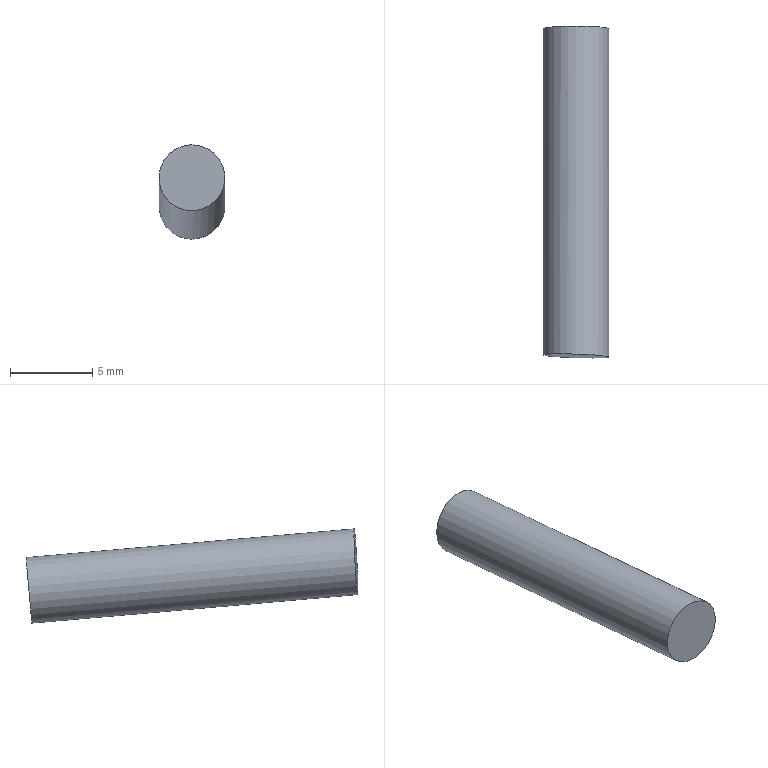Part | NX | features solid 2 | 1 solid | 3 faces | box 4 x 20.154 x 5.728 mm | volume 250.481 mm3 | plane 2 | cylinder 1 | commonest cylinder face diameters 4 x1
STEP:
#1=CARTESIAN_POINT('',(398.525,-42.176,-27.83));
#2=VERTEX_POINT('',#1);
#3=CARTESIAN_POINT('',(398.525,-42.35,-29.823));
#4=DIRECTION('',(0.,0.9962,-0.08716));
#5=DIRECTION('',(0.,0.08716,0.9962));
#6=AXIS2_PLACEMENT_3D('',#3,#4,#5);
#7=CIRCLE('',#6,2.);
#8=EDGE_CURVE('',#2,#2,#7,.F.);
#9=ORIENTED_EDGE('',*,*,#8,.F.);
#10=EDGE_LOOP('',(#9));
#11=FACE_BOUND('',#10,.T.);
#12=CARTESIAN_POINT('',(398.525,-43.44,-42.275));
#13=DIRECTION('',(0.,0.9962,-0.08716));
#14=DIRECTION('',(0.,0.08716,0.9962));
#15=AXIS2_PLACEMENT_3D('',#12,#13,#14);
#16=PLANE('',#15);
#17=ADVANCED_FACE('',(#11),#16,.T.);
#18=CARTESIAN_POINT('',(397.185,-62.246,-29.573));
#19=VERTEX_POINT('',#18);
#20=CARTESIAN_POINT('',(398.525,-62.207,-28.086));
#21=DIRECTION('',(0.03046,0.9981,-0.05344));
#22=DIRECTION('',(-0.6692,-0.01935,-0.7428));
#23=AXIS2_PLACEMENT_3D('',#20,#21,#22);
#24=ELLIPSE('',#23,2.002,2.);
#25=EDGE_CURVE('',#19,#19,#24,.T.);
#26=ORIENTED_EDGE('',*,*,#25,.F.);
#27=EDGE_LOOP('',(#26));
#28=FACE_BOUND('',#27,.T.);
#29=CARTESIAN_POINT('',(457.994,-68.531,-112.302));
#30=DIRECTION('',(0.03046,0.9981,-0.05344));
#31=DIRECTION('',(0.06614,0.05134,0.9965));
#32=AXIS2_PLACEMENT_3D('',#29,#30,#31);
#33=PLANE('',#32);
#34=ADVANCED_FACE('',(#28),#33,.F.);
#35=ORIENTED_EDGE('',*,*,#8,.T.);
#36=EDGE_LOOP('',(#35));
#37=FACE_BOUND('',#36,.T.);
#38=ORIENTED_EDGE('',*,*,#25,.T.);
#39=EDGE_LOOP('',(#38));
#40=FACE_BOUND('',#39,.T.);
#41=CARTESIAN_POINT('',(398.525,-64.267,-27.905));
#42=DIRECTION('',(0.,0.9962,-0.08716));
#43=DIRECTION('',(0.,0.08716,0.9962));
#44=AXIS2_PLACEMENT_3D('',#41,#42,#43);
#45=CYLINDRICAL_SURFACE('',#44,2.);
#46=ADVANCED_FACE('',(#37,#40),#45,.T.);
#47=CLOSED_SHELL('',(#17,#34,#46));
#48=MANIFOLD_SOLID_BREP('',#47);
#49=(LENGTH_UNIT()NAMED_UNIT(*)SI_UNIT(.MILLI.,.METRE.));
#50=UNCERTAINTY_MEASURE_WITH_UNIT(LENGTH_MEASURE(0.00001),#49,'','');
#51=(NAMED_UNIT(*)PLANE_ANGLE_UNIT()SI_UNIT($,.RADIAN.));
#52=(NAMED_UNIT(*)SI_UNIT($,.STERADIAN.)SOLID_ANGLE_UNIT());
#53=(GEOMETRIC_REPRESENTATION_CONTEXT(3)GLOBAL_UNCERTAINTY_ASSIGNED_CONTEXT((#50))GLOBAL_UNIT_ASSIGNED_CONTEXT((#49,#51,#52))REPRESENTATION_CONTEXT('',''));
#54=ADVANCED_BREP_SHAPE_REPRESENTATION('',(#48),#53);